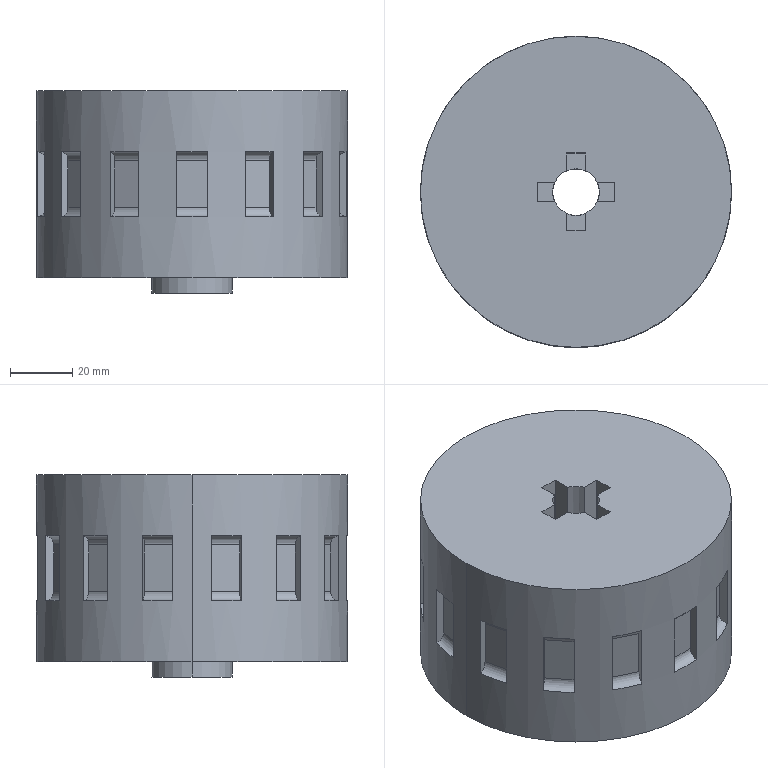Part | SolidWorks | features ICE 2, CirPattern 1, Extrusion 1 | 1 solid | 95 faces | box 100 x 100 x 65 mm | volume 446877 mm3 | plane 61 | cylinder 34 | commonest cylinder face diameters 6 x28 15 x2 26 x2 100 x2